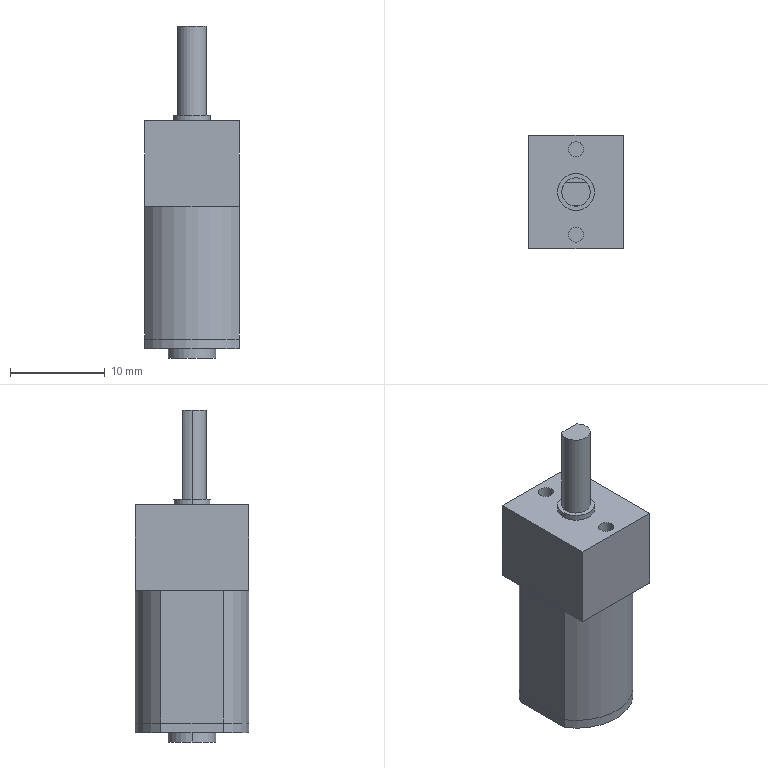Part | SolidWorks | features MBimport 1 | 4 solids | 39 faces | box 10 x 12 x 35 mm | volume 2719 mm3 | plane 23 | cylinder 16 | commonest cylinder face diameters 1.6 x4 3 x4 12 x4 3.9 x2 5 x2
STEP:
#1=CARTESIAN_POINT('',(5.,3.317,-14.));
#2=VERTEX_POINT('',#1);
#3=CARTESIAN_POINT('',(5.,-3.317,-14.));
#4=VERTEX_POINT('',#3);
#5=CARTESIAN_POINT('',(5.,1.658,-14.));
#6=DIRECTION('',(0.,-1.,0.));
#7=VECTOR('',#6,1000.);
#8=LINE('',#5,#7);
#9=EDGE_CURVE('',#2,#4,#8,.T.);
#10=ORIENTED_EDGE('',*,*,#9,.T.);
#11=CARTESIAN_POINT('',(-5.,-3.317,-14.));
#12=VERTEX_POINT('',#11);
#13=CARTESIAN_POINT('',(0.,0.,-14.));
#14=DIRECTION('',(0.,0.,-1.));
#15=DIRECTION('',(1.,0.,0.));
#16=AXIS2_PLACEMENT_3D('',#13,#14,#15);
#17=CIRCLE('',#16,6.);
#18=EDGE_CURVE('',#4,#12,#17,.T.);
#19=ORIENTED_EDGE('',*,*,#18,.T.);
#20=CARTESIAN_POINT('',(-5.,3.317,-14.));
#21=VERTEX_POINT('',#20);
#22=CARTESIAN_POINT('',(-5.,-1.658,-14.));
#23=DIRECTION('',(0.,1.,0.));
#24=VECTOR('',#23,1000.);
#25=LINE('',#22,#24);
#26=EDGE_CURVE('',#12,#21,#25,.T.);
#27=ORIENTED_EDGE('',*,*,#26,.T.);
#28=CARTESIAN_POINT('',(0.,0.,-14.));
#29=DIRECTION('',(0.,0.,-1.));
#30=DIRECTION('',(1.,0.,0.));
#31=AXIS2_PLACEMENT_3D('',#28,#29,#30);
#32=CIRCLE('',#31,6.);
#33=EDGE_CURVE('',#21,#2,#32,.T.);
#34=ORIENTED_EDGE('',*,*,#33,.T.);
#35=EDGE_LOOP('',(#10,#19,#27,#34));
#36=FACE_OUTER_BOUND('',#35,.T.);
#37=CARTESIAN_POINT('',(0.,0.,-14.));
#38=DIRECTION('',(0.,0.,-1.));
#39=DIRECTION('',(0.,-1.,0.));
#40=AXIS2_PLACEMENT_3D('',#37,#38,#39);
#41=PLANE('',#40);
#42=ADVANCED_FACE('',(#36),#41,.T.);
#43=ORIENTED_EDGE('',*,*,#18,.F.);
#44=CARTESIAN_POINT('',(5.,-3.317,0.));
#45=VERTEX_POINT('',#44);
#46=CARTESIAN_POINT('',(5.,-3.317,0.));
#47=DIRECTION('',(0.,0.,-1.));
#48=VECTOR('',#47,1000.);
#49=LINE('',#46,#48);
#50=EDGE_CURVE('',#45,#4,#49,.T.);
#51=ORIENTED_EDGE('',*,*,#50,.F.);
#52=CARTESIAN_POINT('',(-5.,-3.317,0.));
#53=VERTEX_POINT('',#52);
#54=CARTESIAN_POINT('',(0.,0.,0.));
#55=DIRECTION('',(0.,0.,1.));
#56=DIRECTION('',(1.,0.,0.));
#57=AXIS2_PLACEMENT_3D('',#54,#55,#56);
#58=CIRCLE('',#57,6.);
#59=EDGE_CURVE('',#53,#45,#58,.T.);
#60=ORIENTED_EDGE('',*,*,#59,.F.);
#61=CARTESIAN_POINT('',(-5.,-3.317,0.));
#62=DIRECTION('',(0.,0.,-1.));
#63=VECTOR('',#62,1000.);
#64=LINE('',#61,#63);
#65=EDGE_CURVE('',#53,#12,#64,.T.);
#66=ORIENTED_EDGE('',*,*,#65,.T.);
#67=EDGE_LOOP('',(#43,#51,#60,#66));
#68=FACE_OUTER_BOUND('',#67,.T.);
#69=CARTESIAN_POINT('',(0.,0.,0.));
#70=DIRECTION('',(0.,0.,-1.));
#71=DIRECTION('',(1.,0.,0.));
#72=AXIS2_PLACEMENT_3D('',#69,#70,#71);
#73=CYLINDRICAL_SURFACE('',#72,6.);
#74=ADVANCED_FACE('',(#68),#73,.T.);
#75=ORIENTED_EDGE('',*,*,#9,.F.);
#76=CARTESIAN_POINT('',(5.,3.317,0.));
#77=VERTEX_POINT('',#76);
#78=CARTESIAN_POINT('',(5.,3.317,0.));
#79=DIRECTION('',(0.,0.,-1.));
#80=VECTOR('',#79,1000.);
#81=LINE('',#78,#80);
#82=EDGE_CURVE('',#77,#2,#81,.T.);
#83=ORIENTED_EDGE('',*,*,#82,.F.);
#84=CARTESIAN_POINT('',(5.,6.,0.));
#85=DIRECTION('',(0.,-1.,0.));
#86=VECTOR('',#85,1000.);
#87=LINE('',#84,#86);
#88=EDGE_CURVE('',#77,#45,#87,.T.);
#89=ORIENTED_EDGE('',*,*,#88,.T.);
#90=ORIENTED_EDGE('',*,*,#50,.T.);
#91=EDGE_LOOP('',(#75,#83,#89,#90));
#92=FACE_OUTER_BOUND('',#91,.T.);
#93=CARTESIAN_POINT('',(5.,3.317,0.));
#94=DIRECTION('',(1.,0.,0.));
#95=DIRECTION('',(0.,1.,0.));
#96=AXIS2_PLACEMENT_3D('',#93,#94,#95);
#97=PLANE('',#96);
#98=ADVANCED_FACE('',(#92),#97,.T.);
#99=ORIENTED_EDGE('',*,*,#33,.F.);
#100=CARTESIAN_POINT('',(-5.,3.317,0.));
#101=VERTEX_POINT('',#100);
#102=CARTESIAN_POINT('',(-5.,3.317,0.));
#103=DIRECTION('',(0.,0.,-1.));
#104=VECTOR('',#103,1000.);
#105=LINE('',#102,#104);
#106=EDGE_CURVE('',#101,#21,#105,.T.);
#107=ORIENTED_EDGE('',*,*,#106,.F.);
#108=CARTESIAN_POINT('',(0.,0.,0.));
#109=DIRECTION('',(0.,0.,1.));
#110=DIRECTION('',(1.,0.,0.));
#111=AXIS2_PLACEMENT_3D('',#108,#109,#110);
#112=CIRCLE('',#111,6.);
#113=EDGE_CURVE('',#77,#101,#112,.T.);
#114=ORIENTED_EDGE('',*,*,#113,.F.);
#115=ORIENTED_EDGE('',*,*,#82,.T.);
#116=EDGE_LOOP('',(#99,#107,#114,#115));
#117=FACE_OUTER_BOUND('',#116,.T.);
#118=CARTESIAN_POINT('',(0.,0.,0.));
#119=DIRECTION('',(0.,0.,-1.));
#120=DIRECTION('',(1.,0.,0.));
#121=AXIS2_PLACEMENT_3D('',#118,#119,#120);
#122=CYLINDRICAL_SURFACE('',#121,6.);
#123=ADVANCED_FACE('',(#117),#122,.T.);
#124=ORIENTED_EDGE('',*,*,#26,.F.);
#125=ORIENTED_EDGE('',*,*,#65,.F.);
#126=CARTESIAN_POINT('',(-5.,-6.,0.));
#127=DIRECTION('',(0.,1.,0.));
#128=VECTOR('',#127,1000.);
#129=LINE('',#126,#128);
#130=EDGE_CURVE('',#53,#101,#129,.T.);
#131=ORIENTED_EDGE('',*,*,#130,.T.);
#132=ORIENTED_EDGE('',*,*,#106,.T.);
#133=EDGE_LOOP('',(#124,#125,#131,#132));
#134=FACE_OUTER_BOUND('',#133,.T.);
#135=CARTESIAN_POINT('',(-5.,-3.317,0.));
#136=DIRECTION('',(-1.,0.,0.));
#137=DIRECTION('',(0.,0.,1.));
#138=AXIS2_PLACEMENT_3D('',#135,#136,#137);
#139=PLANE('',#138);
#140=ADVANCED_FACE('',(#134),#139,.T.);
#141=ORIENTED_EDGE('',*,*,#59,.T.);
#142=ORIENTED_EDGE('',*,*,#88,.F.);
#143=ORIENTED_EDGE('',*,*,#113,.T.);
#144=ORIENTED_EDGE('',*,*,#130,.F.);
#145=EDGE_LOOP('',(#141,#142,#143,#144));
#146=FACE_OUTER_BOUND('',#145,.T.);
#147=CARTESIAN_POINT('',(0.,0.,0.));
#148=DIRECTION('',(0.,0.,1.));
#149=DIRECTION('',(1.,0.,0.));
#150=AXIS2_PLACEMENT_3D('',#147,#148,#149);
#151=PLANE('',#150);
#152=ADVANCED_FACE('',(#146),#151,.T.);
#153=CLOSED_SHELL('',(#42,#74,#98,#123,#140,#152));
#154=MANIFOLD_SOLID_BREP('',#153);
#155=CARTESIAN_POINT('',(1.5,0.,9.));
#156=VERTEX_POINT('',#155);
#157=CARTESIAN_POINT('',(-1.5,0.,9.));
#158=VERTEX_POINT('',#157);
#159=CARTESIAN_POINT('',(0.,0.,9.));
#160=DIRECTION('',(0.,0.,1.));
#161=DIRECTION('',(1.,0.,0.));
#162=AXIS2_PLACEMENT_3D('',#159,#160,#161);
#163=CIRCLE('',#162,1.5);
#164=EDGE_CURVE('',#156,#158,#163,.T.);
#165=ORIENTED_EDGE('',*,*,#164,.T.);
#166=CARTESIAN_POINT('',(-1.5,0.,19.));
#167=VERTEX_POINT('',#166);
#168=CARTESIAN_POINT('',(-1.5,0.,9.));
#169=DIRECTION('',(0.,0.,1.));
#170=VECTOR('',#169,1000.);
#171=LINE('',#168,#170);
#172=EDGE_CURVE('',#158,#167,#171,.T.);
#173=ORIENTED_EDGE('',*,*,#172,.T.);
#174=CARTESIAN_POINT('',(-1.118,1.,19.));
#175=VERTEX_POINT('',#174);
#176=CARTESIAN_POINT('',(0.,0.,19.));
#177=DIRECTION('',(0.,0.,1.));
#178=DIRECTION('',(1.,0.,0.));
#179=AXIS2_PLACEMENT_3D('',#176,#177,#178);
#180=CIRCLE('',#179,1.5);
#181=EDGE_CURVE('',#175,#167,#180,.T.);
#182=ORIENTED_EDGE('',*,*,#181,.F.);
#183=CARTESIAN_POINT('',(-1.118,1.,9.6));
#184=VERTEX_POINT('',#183);
#185=CARTESIAN_POINT('',(-1.118,1.,9.));
#186=DIRECTION('',(0.,0.,1.));
#187=VECTOR('',#186,1000.);
#188=LINE('',#185,#187);
#189=EDGE_CURVE('',#184,#175,#188,.T.);
#190=ORIENTED_EDGE('',*,*,#189,.F.);
#191=CARTESIAN_POINT('',(1.118,1.,9.6));
#192=VERTEX_POINT('',#191);
#193=CARTESIAN_POINT('',(0.,0.,9.6));
#194=DIRECTION('',(0.,0.,1.));
#195=DIRECTION('',(1.,0.,0.));
#196=AXIS2_PLACEMENT_3D('',#193,#194,#195);
#197=CIRCLE('',#196,1.5);
#198=EDGE_CURVE('',#192,#184,#197,.T.);
#199=ORIENTED_EDGE('',*,*,#198,.F.);
#200=CARTESIAN_POINT('',(1.118,1.,19.));
#201=VERTEX_POINT('',#200);
#202=CARTESIAN_POINT('',(1.118,1.,9.));
#203=DIRECTION('',(0.,0.,1.));
#204=VECTOR('',#203,1000.);
#205=LINE('',#202,#204);
#206=EDGE_CURVE('',#192,#201,#205,.T.);
#207=ORIENTED_EDGE('',*,*,#206,.T.);
#208=CARTESIAN_POINT('',(1.5,0.,19.));
#209=VERTEX_POINT('',#208);
#210=CARTESIAN_POINT('',(0.,0.,19.));
#211=DIRECTION('',(0.,0.,1.));
#212=DIRECTION('',(1.,0.,0.));
#213=AXIS2_PLACEMENT_3D('',#210,#211,#212);
#214=CIRCLE('',#213,1.5);
#215=EDGE_CURVE('',#209,#201,#214,.T.);
#216=ORIENTED_EDGE('',*,*,#215,.F.);
#217=CARTESIAN_POINT('',(1.5,0.,9.));
#218=DIRECTION('',(0.,0.,1.));
#219=VECTOR('',#218,1000.);
#220=LINE('',#217,#219);
#221=EDGE_CURVE('',#156,#209,#220,.T.);
#222=ORIENTED_EDGE('',*,*,#221,.F.);
#223=EDGE_LOOP('',(#165,#173,#182,#190,#199,#207,#216,#222));
#224=FACE_OUTER_BOUND('',#223,.T.);
#225=CARTESIAN_POINT('',(0.,0.,9.));
#226=DIRECTION('',(0.,0.,1.));
#227=DIRECTION('',(1.,0.,0.));
#228=AXIS2_PLACEMENT_3D('',#225,#226,#227);
#229=CYLINDRICAL_SURFACE('',#228,1.5);
#230=ADVANCED_FACE('',(#224),#229,.T.);
#231=ORIENTED_EDGE('',*,*,#164,.F.);
#232=CARTESIAN_POINT('',(0.,0.,9.));
#233=DIRECTION('',(0.,0.,1.));
#234=DIRECTION('',(1.,0.,0.));
#235=AXIS2_PLACEMENT_3D('',#232,#233,#234);
#236=CIRCLE('',#235,1.5);
#237=EDGE_CURVE('',#158,#156,#236,.T.);
#238=ORIENTED_EDGE('',*,*,#237,.F.);
#239=EDGE_LOOP('',(#231,#238));
#240=FACE_OUTER_BOUND('',#239,.T.);
#241=CARTESIAN_POINT('',(0.,1.25,9.));
#242=DIRECTION('',(0.,0.,1.));
#243=DIRECTION('',(1.,0.,0.));
#244=AXIS2_PLACEMENT_3D('',#241,#242,#243);
#245=PLANE('',#244);
#246=ADVANCED_FACE('',(#240),#245,.F.);
#247=ORIENTED_EDGE('',*,*,#198,.T.);
#248=CARTESIAN_POINT('',(1.118,1.,9.6));
#249=DIRECTION('',(1.,0.,0.));
#250=VECTOR('',#249,1000.);
#251=LINE('',#248,#250);
#252=EDGE_CURVE('',#184,#192,#251,.T.);
#253=ORIENTED_EDGE('',*,*,#252,.T.);
#254=EDGE_LOOP('',(#247,#253));
#255=FACE_OUTER_BOUND('',#254,.T.);
#256=CARTESIAN_POINT('',(0.,1.25,9.6));
#257=DIRECTION('',(0.,0.,1.));
#258=DIRECTION('',(1.,0.,0.));
#259=AXIS2_PLACEMENT_3D('',#256,#257,#258);
#260=PLANE('',#259);
#261=ADVANCED_FACE('',(#255),#260,.T.);
#262=ORIENTED_EDGE('',*,*,#172,.F.);
#263=ORIENTED_EDGE('',*,*,#237,.T.);
#264=ORIENTED_EDGE('',*,*,#221,.T.);
#265=CARTESIAN_POINT('',(0.,0.,19.));
#266=DIRECTION('',(0.,0.,1.));
#267=DIRECTION('',(1.,0.,0.));
#268=AXIS2_PLACEMENT_3D('',#265,#266,#267);
#269=CIRCLE('',#268,1.5);
#270=EDGE_CURVE('',#167,#209,#269,.T.);
#271=ORIENTED_EDGE('',*,*,#270,.F.);
#272=EDGE_LOOP('',(#262,#263,#264,#271));
#273=FACE_OUTER_BOUND('',#272,.T.);
#274=CARTESIAN_POINT('',(0.,0.,9.));
#275=DIRECTION('',(0.,0.,1.));
#276=DIRECTION('',(1.,0.,0.));
#277=AXIS2_PLACEMENT_3D('',#274,#275,#276);
#278=CYLINDRICAL_SURFACE('',#277,1.5);
#279=ADVANCED_FACE('',(#273),#278,.T.);
#280=CARTESIAN_POINT('',(1.118,1.,19.));
#281=DIRECTION('',(-1.,0.,0.));
#282=VECTOR('',#281,1000.);
#283=LINE('',#280,#282);
#284=EDGE_CURVE('',#201,#175,#283,.T.);
#285=ORIENTED_EDGE('',*,*,#284,.T.);
#286=ORIENTED_EDGE('',*,*,#181,.T.);
#287=ORIENTED_EDGE('',*,*,#270,.T.);
#288=ORIENTED_EDGE('',*,*,#215,.T.);
#289=EDGE_LOOP('',(#285,#286,#287,#288));
#290=FACE_OUTER_BOUND('',#289,.T.);
#291=CARTESIAN_POINT('',(0.,-0.25,19.));
#292=DIRECTION('',(0.,0.,1.));
#293=DIRECTION('',(1.,0.,0.));
#294=AXIS2_PLACEMENT_3D('',#291,#292,#293);
#295=PLANE('',#294);
#296=ADVANCED_FACE('',(#290),#295,.T.);
#297=ORIENTED_EDGE('',*,*,#252,.F.);
#298=ORIENTED_EDGE('',*,*,#189,.T.);
#299=ORIENTED_EDGE('',*,*,#284,.F.);
#300=ORIENTED_EDGE('',*,*,#206,.F.);
#301=EDGE_LOOP('',(#297,#298,#299,#300));
#302=FACE_OUTER_BOUND('',#301,.T.);
#303=CARTESIAN_POINT('',(1.118,1.,9.));
#304=DIRECTION('',(0.,1.,0.));
#305=DIRECTION('',(1.,0.,0.));
#306=AXIS2_PLACEMENT_3D('',#303,#304,#305);
#307=PLANE('',#306);
#308=ADVANCED_FACE('',(#302),#307,.T.);
#309=CLOSED_SHELL('',(#230,#246,#261,#279,#296,#308));
#310=MANIFOLD_SOLID_BREP('',#309);
#311=CARTESIAN_POINT('',(2.5,0.,-15.));
#312=VERTEX_POINT('',#311);
#313=CARTESIAN_POINT('',(-2.5,0.,-15.));
#314=VERTEX_POINT('',#313);
#315=CARTESIAN_POINT('',(0.,0.,-15.));
#316=DIRECTION('',(0.,0.,1.));
#317=DIRECTION('',(-1.,0.,0.));
#318=AXIS2_PLACEMENT_3D('',#315,#316,#317);
#319=CIRCLE('',#318,2.5);
#320=EDGE_CURVE('',#312,#314,#319,.T.);
#321=ORIENTED_EDGE('',*,*,#320,.F.);
#322=CARTESIAN_POINT('',(2.5,0.,-16.));
#323=VERTEX_POINT('',#322);
#324=CARTESIAN_POINT('',(2.5,0.,-15.));
#325=DIRECTION('',(0.,0.,-1.));
#326=VECTOR('',#325,1000.);
#327=LINE('',#324,#326);
#328=EDGE_CURVE('',#312,#323,#327,.T.);
#329=ORIENTED_EDGE('',*,*,#328,.T.);
#330=CARTESIAN_POINT('',(-2.5,0.,-16.));
#331=VERTEX_POINT('',#330);
#332=CARTESIAN_POINT('',(0.,0.,-16.));
#333=DIRECTION('',(0.,0.,-1.));
#334=DIRECTION('',(-1.,0.,0.));
#335=AXIS2_PLACEMENT_3D('',#332,#333,#334);
#336=CIRCLE('',#335,2.5);
#337=EDGE_CURVE('',#331,#323,#336,.T.);
#338=ORIENTED_EDGE('',*,*,#337,.F.);
#339=CARTESIAN_POINT('',(-2.5,0.,-15.));
#340=DIRECTION('',(0.,0.,-1.));
#341=VECTOR('',#340,1000.);
#342=LINE('',#339,#341);
#343=EDGE_CURVE('',#314,#331,#342,.T.);
#344=ORIENTED_EDGE('',*,*,#343,.F.);
#345=EDGE_LOOP('',(#321,#329,#338,#344));
#346=FACE_OUTER_BOUND('',#345,.T.);
#347=CARTESIAN_POINT('',(0.,0.,-15.));
#348=DIRECTION('',(0.,0.,-1.));
#349=DIRECTION('',(-1.,0.,0.));
#350=AXIS2_PLACEMENT_3D('',#347,#348,#349);
#351=CYLINDRICAL_SURFACE('',#350,2.5);
#352=ADVANCED_FACE('',(#346),#351,.T.);
#353=CARTESIAN_POINT('',(0.,0.,-15.));
#354=DIRECTION('',(0.,0.,1.));
#355=DIRECTION('',(-1.,0.,0.));
#356=AXIS2_PLACEMENT_3D('',#353,#354,#355);
#357=CIRCLE('',#356,2.5);
#358=EDGE_CURVE('',#314,#312,#357,.T.);
#359=ORIENTED_EDGE('',*,*,#358,.T.);
#360=ORIENTED_EDGE('',*,*,#320,.T.);
#361=EDGE_LOOP('',(#359,#360));
#362=FACE_BOUND('',#361,.T.);
#363=CARTESIAN_POINT('',(5.,-3.317,-15.));
#364=VERTEX_POINT('',#363);
#365=CARTESIAN_POINT('',(-5.,-3.317,-15.));
#366=VERTEX_POINT('',#365);
#367=CARTESIAN_POINT('',(0.,0.,-15.));
#368=DIRECTION('',(0.,0.,-1.));
#369=DIRECTION('',(1.,0.,0.));
#370=AXIS2_PLACEMENT_3D('',#367,#368,#369);
#371=CIRCLE('',#370,6.);
#372=EDGE_CURVE('',#364,#366,#371,.T.);
#373=ORIENTED_EDGE('',*,*,#372,.T.);
#374=CARTESIAN_POINT('',(-5.,3.317,-15.));
#375=VERTEX_POINT('',#374);
#376=CARTESIAN_POINT('',(-5.,-6.,-15.));
#377=DIRECTION('',(0.,1.,0.));
#378=VECTOR('',#377,1000.);
#379=LINE('',#376,#378);
#380=EDGE_CURVE('',#366,#375,#379,.T.);
#381=ORIENTED_EDGE('',*,*,#380,.T.);
#382=CARTESIAN_POINT('',(5.,3.317,-15.));
#383=VERTEX_POINT('',#382);
#384=CARTESIAN_POINT('',(0.,0.,-15.));
#385=DIRECTION('',(0.,0.,-1.));
#386=DIRECTION('',(1.,0.,0.));
#387=AXIS2_PLACEMENT_3D('',#384,#385,#386);
#388=CIRCLE('',#387,6.);
#389=EDGE_CURVE('',#375,#383,#388,.T.);
#390=ORIENTED_EDGE('',*,*,#389,.T.);
#391=CARTESIAN_POINT('',(5.,6.,-15.));
#392=DIRECTION('',(0.,-1.,0.));
#393=VECTOR('',#392,1000.);
#394=LINE('',#391,#393);
#395=EDGE_CURVE('',#383,#364,#394,.T.);
#396=ORIENTED_EDGE('',*,*,#395,.T.);
#397=EDGE_LOOP('',(#373,#381,#390,#396));
#398=FACE_OUTER_BOUND('',#397,.T.);
#399=CARTESIAN_POINT('',(0.,0.,-15.));
#400=DIRECTION('',(0.,0.,1.));
#401=DIRECTION('',(1.,0.,0.));
#402=AXIS2_PLACEMENT_3D('',#399,#400,#401);
#403=PLANE('',#402);
#404=ADVANCED_FACE('',(#362,#398),#403,.F.);
#405=CARTESIAN_POINT('',(5.,-3.317,-14.));
#406=VERTEX_POINT('',#405);
#407=CARTESIAN_POINT('',(-5.,-3.317,-14.));
#408=VERTEX_POINT('',#407);
#409=CARTESIAN_POINT('',(0.,0.,-14.));
#410=DIRECTION('',(0.,0.,-1.));
#411=DIRECTION('',(1.,0.,0.));
#412=AXIS2_PLACEMENT_3D('',#409,#410,#411);
#413=CIRCLE('',#412,6.);
#414=EDGE_CURVE('',#406,#408,#413,.T.);
#415=ORIENTED_EDGE('',*,*,#414,.T.);
#416=CARTESIAN_POINT('',(-5.,-3.317,0.));
#417=DIRECTION('',(0.,0.,-1.));
#418=VECTOR('',#417,1000.);
#419=LINE('',#416,#418);
#420=EDGE_CURVE('',#408,#366,#419,.T.);
#421=ORIENTED_EDGE('',*,*,#420,.T.);
#422=ORIENTED_EDGE('',*,*,#372,.F.);
#423=CARTESIAN_POINT('',(5.,-3.317,0.));
#424=DIRECTION('',(0.,0.,-1.));
#425=VECTOR('',#424,1000.);
#426=LINE('',#423,#425);
#427=EDGE_CURVE('',#406,#364,#426,.T.);
#428=ORIENTED_EDGE('',*,*,#427,.F.);
#429=EDGE_LOOP('',(#415,#421,#422,#428));
#430=FACE_OUTER_BOUND('',#429,.T.);
#431=CARTESIAN_POINT('',(0.,0.,0.));
#432=DIRECTION('',(0.,0.,-1.));
#433=DIRECTION('',(1.,0.,0.));
#434=AXIS2_PLACEMENT_3D('',#431,#432,#433);
#435=CYLINDRICAL_SURFACE('',#434,6.);
#436=ADVANCED_FACE('',(#430),#435,.T.);
#437=CARTESIAN_POINT('',(5.,3.317,-14.));
#438=VERTEX_POINT('',#437);
#439=CARTESIAN_POINT('',(5.,1.658,-14.));
#440=DIRECTION('',(0.,-1.,0.));
#441=VECTOR('',#440,1000.);
#442=LINE('',#439,#441);
#443=EDGE_CURVE('',#438,#406,#442,.T.);
#444=ORIENTED_EDGE('',*,*,#443,.T.);
#445=ORIENTED_EDGE('',*,*,#427,.T.);
#446=ORIENTED_EDGE('',*,*,#395,.F.);
#447=CARTESIAN_POINT('',(5.,3.317,0.));
#448=DIRECTION('',(0.,0.,-1.));
#449=VECTOR('',#448,1000.);
#450=LINE('',#447,#449);
#451=EDGE_CURVE('',#438,#383,#450,.T.);
#452=ORIENTED_EDGE('',*,*,#451,.F.);
#453=EDGE_LOOP('',(#444,#445,#446,#452));
#454=FACE_OUTER_BOUND('',#453,.T.);
#455=CARTESIAN_POINT('',(5.,3.317,0.));
#456=DIRECTION('',(1.,0.,0.));
#457=DIRECTION('',(0.,1.,0.));
#458=AXIS2_PLACEMENT_3D('',#455,#456,#457);
#459=PLANE('',#458);
#460=ADVANCED_FACE('',(#454),#459,.T.);
#461=ORIENTED_EDGE('',*,*,#337,.T.);
#462=CARTESIAN_POINT('',(0.,0.,-16.));
#463=DIRECTION('',(0.,0.,-1.));
#464=DIRECTION('',(-1.,0.,0.));
#465=AXIS2_PLACEMENT_3D('',#462,#463,#464);
#466=CIRCLE('',#465,2.5);
#467=EDGE_CURVE('',#323,#331,#466,.T.);
#468=ORIENTED_EDGE('',*,*,#467,.T.);
#469=EDGE_LOOP('',(#461,#468));
#470=FACE_OUTER_BOUND('',#469,.T.);
#471=CARTESIAN_POINT('',(0.,0.,-16.));
#472=DIRECTION('',(0.,0.,-1.));
#473=DIRECTION('',(0.,-1.,0.));
#474=AXIS2_PLACEMENT_3D('',#471,#472,#473);
#475=PLANE('',#474);
#476=ADVANCED_FACE('',(#470),#475,.T.);
#477=ORIENTED_EDGE('',*,*,#328,.F.);
#478=ORIENTED_EDGE('',*,*,#358,.F.);
#479=ORIENTED_EDGE('',*,*,#343,.T.);
#480=ORIENTED_EDGE('',*,*,#467,.F.);
#481=EDGE_LOOP('',(#477,#478,#479,#480));
#482=FACE_OUTER_BOUND('',#481,.T.);
#483=CARTESIAN_POINT('',(0.,0.,-15.));
#484=DIRECTION('',(0.,0.,-1.));
#485=DIRECTION('',(-1.,0.,0.));
#486=AXIS2_PLACEMENT_3D('',#483,#484,#485);
#487=CYLINDRICAL_SURFACE('',#486,2.5);
#488=ADVANCED_FACE('',(#482),#487,.T.);
#489=CARTESIAN_POINT('',(-5.,3.317,-14.));
#490=VERTEX_POINT('',#489);
#491=CARTESIAN_POINT('',(0.,0.,-14.));
#492=DIRECTION('',(0.,0.,-1.));
#493=DIRECTION('',(1.,0.,0.));
#494=AXIS2_PLACEMENT_3D('',#491,#492,#493);
#495=CIRCLE('',#494,6.);
#496=EDGE_CURVE('',#490,#438,#495,.T.);
#497=ORIENTED_EDGE('',*,*,#496,.T.);
#498=ORIENTED_EDGE('',*,*,#451,.T.);
#499=ORIENTED_EDGE('',*,*,#389,.F.);
#500=CARTESIAN_POINT('',(-5.,3.317,0.));
#501=DIRECTION('',(0.,0.,-1.));
#502=VECTOR('',#501,1000.);
#503=LINE('',#500,#502);
#504=EDGE_CURVE('',#490,#375,#503,.T.);
#505=ORIENTED_EDGE('',*,*,#504,.F.);
#506=EDGE_LOOP('',(#497,#498,#499,#505));
#507=FACE_OUTER_BOUND('',#506,.T.);
#508=CARTESIAN_POINT('',(0.,0.,0.));
#509=DIRECTION('',(0.,0.,-1.));
#510=DIRECTION('',(1.,0.,0.));
#511=AXIS2_PLACEMENT_3D('',#508,#509,#510);
#512=CYLINDRICAL_SURFACE('',#511,6.);
#513=ADVANCED_FACE('',(#507),#512,.T.);
#514=CARTESIAN_POINT('',(-5.,-1.658,-14.));
#515=DIRECTION('',(0.,1.,0.));
#516=VECTOR('',#515,1000.);
#517=LINE('',#514,#516);
#518=EDGE_CURVE('',#408,#490,#517,.T.);
#519=ORIENTED_EDGE('',*,*,#518,.T.);
#520=ORIENTED_EDGE('',*,*,#504,.T.);
#521=ORIENTED_EDGE('',*,*,#380,.F.);
#522=ORIENTED_EDGE('',*,*,#420,.F.);
#523=EDGE_LOOP('',(#519,#520,#521,#522));
#524=FACE_OUTER_BOUND('',#523,.T.);
#525=CARTESIAN_POINT('',(-5.,-3.317,0.));
#526=DIRECTION('',(-1.,0.,0.));
#527=DIRECTION('',(0.,0.,1.));
#528=AXIS2_PLACEMENT_3D('',#525,#526,#527);
#529=PLANE('',#528);
#530=ADVANCED_FACE('',(#524),#529,.T.);
#531=ORIENTED_EDGE('',*,*,#443,.F.);
#532=ORIENTED_EDGE('',*,*,#496,.F.);
#533=ORIENTED_EDGE('',*,*,#518,.F.);
#534=ORIENTED_EDGE('',*,*,#414,.F.);
#535=EDGE_LOOP('',(#531,#532,#533,#534));
#536=FACE_OUTER_BOUND('',#535,.T.);
#537=CARTESIAN_POINT('',(0.,0.,-14.));
#538=DIRECTION('',(0.,0.,-1.));
#539=DIRECTION('',(0.,-1.,0.));
#540=AXIS2_PLACEMENT_3D('',#537,#538,#539);
#541=PLANE('',#540);
#542=ADVANCED_FACE('',(#536),#541,.F.);
#543=CLOSED_SHELL('',(#352,#404,#436,#460,#476,#488,#513,#530,#542));
#544=MANIFOLD_SOLID_BREP('',#543);
#545=CARTESIAN_POINT('',(-0.8,4.5,9.));
#546=VERTEX_POINT('',#545);
#547=CARTESIAN_POINT('',(0.8,4.5,9.));
#548=VERTEX_POINT('',#547);
#549=CARTESIAN_POINT('',(0.,4.5,9.));
#550=DIRECTION('',(0.,0.,-1.));
#551=DIRECTION('',(1.,0.,0.));
#552=AXIS2_PLACEMENT_3D('',#549,#550,#551);
#553=CIRCLE('',#552,0.8);
#554=EDGE_CURVE('',#546,#548,#553,.T.);
#555=ORIENTED_EDGE('',*,*,#554,.F.);
#556=CARTESIAN_POINT('',(-0.8,4.5,7.));
#557=VERTEX_POINT('',#556);
#558=CARTESIAN_POINT('',(-0.8,4.5,9.));
#559=DIRECTION('',(0.,0.,-1.));
#560=VECTOR('',#559,1000.);
#561=LINE('',#558,#560);
#562=EDGE_CURVE('',#546,#557,#561,.T.);
#563=ORIENTED_EDGE('',*,*,#562,.T.);
#564=CARTESIAN_POINT('',(0.8,4.5,7.));
#565=VERTEX_POINT('',#564);
#566=CARTESIAN_POINT('',(0.,4.5,7.));
#567=DIRECTION('',(0.,0.,-1.));
#568=DIRECTION('',(1.,0.,0.));
#569=AXIS2_PLACEMENT_3D('',#566,#567,#568);
#570=CIRCLE('',#569,0.8);
#571=EDGE_CURVE('',#557,#565,#570,.T.);
#572=ORIENTED_EDGE('',*,*,#571,.T.);
#573=CARTESIAN_POINT('',(0.8,4.5,9.));
#574=DIRECTION('',(0.,0.,-1.));
#575=VECTOR('',#574,1000.);
#576=LINE('',#573,#575);
#577=EDGE_CURVE('',#548,#565,#576,.T.);
#578=ORIENTED_EDGE('',*,*,#577,.F.);
#579=EDGE_LOOP('',(#555,#563,#572,#578));
#580=FACE_OUTER_BOUND('',#579,.T.);
#581=CARTESIAN_POINT('',(0.,4.5,9.));
#582=DIRECTION('',(0.,0.,-1.));
#583=DIRECTION('',(1.,0.,0.));
#584=AXIS2_PLACEMENT_3D('',#581,#582,#583);
#585=CYLINDRICAL_SURFACE('',#584,0.8);
#586=ADVANCED_FACE('',(#580),#585,.F.);
#587=CARTESIAN_POINT('',(-0.8,-4.5,9.));
#588=VERTEX_POINT('',#587);
#589=CARTESIAN_POINT('',(0.8,-4.5,9.));
#590=VERTEX_POINT('',#589);
#591=CARTESIAN_POINT('',(0.,-4.5,9.));
#592=DIRECTION('',(0.,0.,-1.));
#593=DIRECTION('',(1.,0.,0.));
#594=AXIS2_PLACEMENT_3D('',#591,#592,#593);
#595=CIRCLE('',#594,0.8);
#596=EDGE_CURVE('',#588,#590,#595,.T.);
#597=ORIENTED_EDGE('',*,*,#596,.F.);
#598=CARTESIAN_POINT('',(-0.8,-4.5,7.));
#599=VERTEX_POINT('',#598);
#600=CARTESIAN_POINT('',(-0.8,-4.5,9.));
#601=DIRECTION('',(0.,0.,-1.));
#602=VECTOR('',#601,1000.);
#603=LINE('',#600,#602);
#604=EDGE_CURVE('',#588,#599,#603,.T.);
#605=ORIENTED_EDGE('',*,*,#604,.T.);
#606=CARTESIAN_POINT('',(0.8,-4.5,7.));
#607=VERTEX_POINT('',#606);
#608=CARTESIAN_POINT('',(0.,-4.5,7.));
#609=DIRECTION('',(0.,0.,-1.));
#610=DIRECTION('',(1.,0.,0.));
#611=AXIS2_PLACEMENT_3D('',#608,#609,#610);
#612=CIRCLE('',#611,0.8);
#613=EDGE_CURVE('',#599,#607,#612,.T.);
#614=ORIENTED_EDGE('',*,*,#613,.T.);
#615=CARTESIAN_POINT('',(0.8,-4.5,9.));
#616=DIRECTION('',(0.,0.,-1.));
#617=VECTOR('',#616,1000.);
#618=LINE('',#615,#617);
#619=EDGE_CURVE('',#590,#607,#618,.T.);
#620=ORIENTED_EDGE('',*,*,#619,.F.);
#621=EDGE_LOOP('',(#597,#605,#614,#620));
#622=FACE_OUTER_BOUND('',#621,.T.);
#623=CARTESIAN_POINT('',(0.,-4.5,9.));
#624=DIRECTION('',(0.,0.,-1.));
#625=DIRECTION('',(1.,0.,0.));
#626=AXIS2_PLACEMENT_3D('',#623,#624,#625);
#627=CYLINDRICAL_SURFACE('',#626,0.8);
#628=ADVANCED_FACE('',(#622),#627,.F.);
#629=CARTESIAN_POINT('',(-1.5,0.,9.));
#630=VERTEX_POINT('',#629);
#631=CARTESIAN_POINT('',(1.5,0.,9.));
#632=VERTEX_POINT('',#631);
#633=CARTESIAN_POINT('',(0.,0.,9.));
#634=DIRECTION('',(0.,0.,1.));
#635=DIRECTION('',(1.,0.,0.));
#636=AXIS2_PLACEMENT_3D('',#633,#634,#635);
#637=CIRCLE('',#636,1.5);
#638=EDGE_CURVE('',#630,#632,#637,.T.);
#639=ORIENTED_EDGE('',*,*,#638,.F.);
#640=CARTESIAN_POINT('',(-1.5,0.,9.6));
#641=VERTEX_POINT('',#640);
#642=CARTESIAN_POINT('',(-1.5,0.,9.));
#643=DIRECTION('',(0.,0.,1.));
#644=VECTOR('',#643,1000.);
#645=LINE('',#642,#644);
#646=EDGE_CURVE('',#630,#641,#645,.T.);
#647=ORIENTED_EDGE('',*,*,#646,.T.);
#648=CARTESIAN_POINT('',(1.5,0.,9.6));
#649=VERTEX_POINT('',#648);
#650=CARTESIAN_POINT('',(0.,0.,9.6));
#651=DIRECTION('',(0.,0.,-1.));
#652=DIRECTION('',(1.,0.,0.));
#653=AXIS2_PLACEMENT_3D('',#650,#651,#652);
#654=CIRCLE('',#653,1.5);
#655=EDGE_CURVE('',#649,#641,#654,.T.);
#656=ORIENTED_EDGE('',*,*,#655,.F.);
#657=CARTESIAN_POINT('',(1.5,0.,9.));
#658=DIRECTION('',(0.,0.,1.));
#659=VECTOR('',#658,1000.);
#660=LINE('',#657,#659);
#661=EDGE_CURVE('',#632,#649,#660,.T.);
#662=ORIENTED_EDGE('',*,*,#661,.F.);
#663=EDGE_LOOP('',(#639,#647,#656,#662));
#664=FACE_OUTER_BOUND('',#663,.T.);
#665=CARTESIAN_POINT('',(0.,0.,9.));
#666=DIRECTION('',(0.,0.,1.));
#667=DIRECTION('',(1.,0.,0.));
#668=AXIS2_PLACEMENT_3D('',#665,#666,#667);
#669=CYLINDRICAL_SURFACE('',#668,1.5);
#670=ADVANCED_FACE('',(#664),#669,.F.);
#671=CARTESIAN_POINT('',(-1.95,0.,9.));
#672=VERTEX_POINT('',#671);
#673=CARTESIAN_POINT('',(1.95,0.,9.));
#674=VERTEX_POINT('',#673);
#675=CARTESIAN_POINT('',(0.,0.,9.));
#676=DIRECTION('',(0.,0.,-1.));
#677=DIRECTION('',(1.,0.,0.));
#678=AXIS2_PLACEMENT_3D('',#675,#676,#677);
#679=CIRCLE('',#678,1.95);
#680=EDGE_CURVE('',#672,#674,#679,.T.);
#681=ORIENTED_EDGE('',*,*,#680,.F.);
#682=CARTESIAN_POINT('',(-1.95,0.,9.6));
#683=VERTEX_POINT('',#682);
#684=CARTESIAN_POINT('',(-1.95,0.,9.));
#685=DIRECTION('',(0.,0.,1.));
#686=VECTOR('',#685,1000.);
#687=LINE('',#684,#686);
#688=EDGE_CURVE('',#672,#683,#687,.T.);
#689=ORIENTED_EDGE('',*,*,#688,.T.);
#690=CARTESIAN_POINT('',(1.95,0.,9.6));
#691=VERTEX_POINT('',#690);
#692=CARTESIAN_POINT('',(0.,0.,9.6));
#693=DIRECTION('',(0.,0.,1.));
#694=DIRECTION('',(1.,0.,0.));
#695=AXIS2_PLACEMENT_3D('',#692,#693,#694);
#696=CIRCLE('',#695,1.95);
#697=EDGE_CURVE('',#691,#683,#696,.T.);
#698=ORIENTED_EDGE('',*,*,#697,.F.);
#699=CARTESIAN_POINT('',(1.95,0.,9.));
#700=DIRECTION('',(0.,0.,1.));
#701=VECTOR('',#700,1000.);
#702=LINE('',#699,#701);
#703=EDGE_CURVE('',#674,#691,#702,.T.);
#704=ORIENTED_EDGE('',*,*,#703,.F.);
#705=EDGE_LOOP('',(#681,#689,#698,#704));
#706=FACE_OUTER_BOUND('',#705,.T.);
#707=CARTESIAN_POINT('',(0.,0.,9.));
#708=DIRECTION('',(0.,0.,1.));
#709=DIRECTION('',(1.,0.,0.));
#710=AXIS2_PLACEMENT_3D('',#707,#708,#709);
#711=CYLINDRICAL_SURFACE('',#710,1.95);
#712=ADVANCED_FACE('',(#706),#711,.T.);
#713=CARTESIAN_POINT('',(5.,-6.,0.));
#714=VERTEX_POINT('',#713);
#715=CARTESIAN_POINT('',(-5.,-6.,0.));
#716=VERTEX_POINT('',#715);
#717=CARTESIAN_POINT('',(5.,-6.,0.));
#718=DIRECTION('',(-1.,0.,0.));
#719=VECTOR('',#718,1000.);
#720=LINE('',#717,#719);
#721=EDGE_CURVE('',#714,#716,#720,.T.);
#722=ORIENTED_EDGE('',*,*,#721,.T.);
#723=CARTESIAN_POINT('',(-5.,6.,0.));
#724=VERTEX_POINT('',#723);
#725=CARTESIAN_POINT('',(-5.,-6.,0.));
#726=DIRECTION('',(0.,1.,0.));
#727=VECTOR('',#726,1000.);
#728=LINE('',#725,#727);
#729=EDGE_CURVE('',#716,#724,#728,.T.);
#730=ORIENTED_EDGE('',*,*,#729,.T.);
#731=CARTESIAN_POINT('',(5.,6.,0.));
#732=VERTEX_POINT('',#731);
#733=CARTESIAN_POINT('',(-5.,6.,0.));
#734=DIRECTION('',(1.,0.,0.));
#735=VECTOR('',#734,1000.);
#736=LINE('',#733,#735);
#737=EDGE_CURVE('',#724,#732,#736,.T.);
#738=ORIENTED_EDGE('',*,*,#737,.T.);
#739=CARTESIAN_POINT('',(5.,6.,0.));
#740=DIRECTION('',(0.,-1.,0.));
#741=VECTOR('',#740,1000.);
#742=LINE('',#739,#741);
#743=EDGE_CURVE('',#732,#714,#742,.T.);
#744=ORIENTED_EDGE('',*,*,#743,.T.);
#745=EDGE_LOOP('',(#722,#730,#738,#744));
#746=FACE_OUTER_BOUND('',#745,.T.);
#747=CARTESIAN_POINT('',(0.,0.,0.));
#748=DIRECTION('',(0.,0.,1.));
#749=DIRECTION('',(1.,0.,0.));
#750=AXIS2_PLACEMENT_3D('',#747,#748,#749);
#751=PLANE('',#750);
#752=ADVANCED_FACE('',(#746),#751,.F.);
#753=CARTESIAN_POINT('',(0.,0.,9.));
#754=DIRECTION('',(0.,0.,1.));
#755=DIRECTION('',(1.,0.,0.));
#756=AXIS2_PLACEMENT_3D('',#753,#754,#755);
#757=CIRCLE('',#756,1.5);
#758=EDGE_CURVE('',#632,#630,#757,.T.);
#759=ORIENTED_EDGE('',*,*,#758,.T.);
#760=ORIENTED_EDGE('',*,*,#638,.T.);
#761=EDGE_LOOP('',(#759,#760));
#762=FACE_OUTER_BOUND('',#761,.T.);
#763=CARTESIAN_POINT('',(0.,0.,9.));
#764=DIRECTION('',(0.,0.,1.));
#765=DIRECTION('',(1.,0.,0.));
#766=AXIS2_PLACEMENT_3D('',#763,#764,#765);
#767=PLANE('',#766);
#768=ADVANCED_FACE('',(#762),#767,.T.);
#769=ORIENTED_EDGE('',*,*,#721,.F.);
#770=CARTESIAN_POINT('',(5.,-6.,9.));
#771=VERTEX_POINT('',#770);
#772=CARTESIAN_POINT('',(5.,-6.,0.));
#773=DIRECTION('',(0.,0.,1.));
#774=VECTOR('',#773,1000.);
#775=LINE('',#772,#774);
#776=EDGE_CURVE('',#714,#771,#775,.T.);
#777=ORIENTED_EDGE('',*,*,#776,.T.);
#778=CARTESIAN_POINT('',(-5.,-6.,9.));
#779=VERTEX_POINT('',#778);
#780=CARTESIAN_POINT('',(5.,-6.,9.));
#781=DIRECTION('',(1.,0.,0.));
#782=VECTOR('',#781,1000.);
#783=LINE('',#780,#782);
#784=EDGE_CURVE('',#779,#771,#783,.T.);
#785=ORIENTED_EDGE('',*,*,#784,.F.);
#786=CARTESIAN_POINT('',(-5.,-6.,0.));
#787=DIRECTION('',(0.,0.,1.));
#788=VECTOR('',#787,1000.);
#789=LINE('',#786,#788);
#790=EDGE_CURVE('',#716,#779,#789,.T.);
#791=ORIENTED_EDGE('',*,*,#790,.F.);
#792=EDGE_LOOP('',(#769,#777,#785,#791));
#793=FACE_OUTER_BOUND('',#792,.T.);
#794=CARTESIAN_POINT('',(-5.,-6.,0.));
#795=DIRECTION('',(0.,-1.,0.));
#796=DIRECTION('',(0.,0.,-1.));
#797=AXIS2_PLACEMENT_3D('',#794,#795,#796);
#798=PLANE('',#797);
#799=ADVANCED_FACE('',(#793),#798,.T.);
#800=ORIENTED_EDGE('',*,*,#743,.F.);
#801=CARTESIAN_POINT('',(5.,6.,9.));
#802=VERTEX_POINT('',#801);
#803=CARTESIAN_POINT('',(5.,6.,0.));
#804=DIRECTION('',(0.,0.,1.));
#805=VECTOR('',#804,1000.);
#806=LINE('',#803,#805);
#807=EDGE_CURVE('',#732,#802,#806,.T.);
#808=ORIENTED_EDGE('',*,*,#807,.T.);
#809=CARTESIAN_POINT('',(5.,6.,9.));
#810=DIRECTION('',(0.,1.,0.));
#811=VECTOR('',#810,1000.);
#812=LINE('',#809,#811);
#813=EDGE_CURVE('',#771,#802,#812,.T.);
#814=ORIENTED_EDGE('',*,*,#813,.F.);
#815=ORIENTED_EDGE('',*,*,#776,.F.);
#816=EDGE_LOOP('',(#800,#808,#814,#815));
#817=FACE_OUTER_BOUND('',#816,.T.);
#818=CARTESIAN_POINT('',(5.,-6.,0.));
#819=DIRECTION('',(1.,0.,0.));
#820=DIRECTION('',(0.,1.,0.));
#821=AXIS2_PLACEMENT_3D('',#818,#819,#820);
#822=PLANE('',#821);
#823=ADVANCED_FACE('',(#817),#822,.T.);
#824=ORIENTED_EDGE('',*,*,#737,.F.);
#825=CARTESIAN_POINT('',(-5.,6.,9.));
#826=VERTEX_POINT('',#825);
#827=CARTESIAN_POINT('',(-5.,6.,0.));
#828=DIRECTION('',(0.,0.,1.));
#829=VECTOR('',#828,1000.);
#830=LINE('',#827,#829);
#831=EDGE_CURVE('',#724,#826,#830,.T.);
#832=ORIENTED_EDGE('',*,*,#831,.T.);
#833=CARTESIAN_POINT('',(-5.,6.,9.));
#834=DIRECTION('',(-1.,0.,0.));
#835=VECTOR('',#834,1000.);
#836=LINE('',#833,#835);
#837=EDGE_CURVE('',#802,#826,#836,.T.);
#838=ORIENTED_EDGE('',*,*,#837,.F.);
#839=ORIENTED_EDGE('',*,*,#807,.F.);
#840=EDGE_LOOP('',(#824,#832,#838,#839));
#841=FACE_OUTER_BOUND('',#840,.T.);
#842=CARTESIAN_POINT('',(5.,6.,0.));
#843=DIRECTION('',(0.,1.,0.));
#844=DIRECTION('',(1.,0.,0.));
#845=AXIS2_PLACEMENT_3D('',#842,#843,#844);
#846=PLANE('',#845);
#847=ADVANCED_FACE('',(#841),#846,.T.);
#848=ORIENTED_EDGE('',*,*,#729,.F.);
#849=ORIENTED_EDGE('',*,*,#790,.T.);
#850=CARTESIAN_POINT('',(-5.,-6.,9.));
#851=DIRECTION('',(0.,-1.,0.));
#852=VECTOR('',#851,1000.);
#853=LINE('',#850,#852);
#854=EDGE_CURVE('',#826,#779,#853,.T.);
#855=ORIENTED_EDGE('',*,*,#854,.F.);
#856=ORIENTED_EDGE('',*,*,#831,.F.);
#857=EDGE_LOOP('',(#848,#849,#855,#856));
#858=FACE_OUTER_BOUND('',#857,.T.);
#859=CARTESIAN_POINT('',(-5.,6.,0.));
#860=DIRECTION('',(-1.,0.,0.));
#861=DIRECTION('',(0.,0.,1.));
#862=AXIS2_PLACEMENT_3D('',#859,#860,#861);
#863=PLANE('',#862);
#864=ADVANCED_FACE('',(#858),#863,.T.);
#865=CARTESIAN_POINT('',(0.,0.,9.));
#866=DIRECTION('',(0.,0.,-1.));
#867=DIRECTION('',(1.,0.,0.));
#868=AXIS2_PLACEMENT_3D('',#865,#866,#867);
#869=CIRCLE('',#868,1.95);
#870=EDGE_CURVE('',#674,#672,#869,.T.);
#871=ORIENTED_EDGE('',*,*,#870,.T.);
#872=ORIENTED_EDGE('',*,*,#680,.T.);
#873=EDGE_LOOP('',(#871,#872));
#874=FACE_BOUND('',#873,.T.);
#875=CARTESIAN_POINT('',(0.,-4.5,9.));
#876=DIRECTION('',(0.,0.,-1.));
#877=DIRECTION('',(1.,0.,0.));
#878=AXIS2_PLACEMENT_3D('',#875,#876,#877);
#879=CIRCLE('',#878,0.8);
#880=EDGE_CURVE('',#590,#588,#879,.T.);
#881=ORIENTED_EDGE('',*,*,#880,.T.);
#882=ORIENTED_EDGE('',*,*,#596,.T.);
#883=EDGE_LOOP('',(#881,#882));
#884=FACE_BOUND('',#883,.T.);
#885=CARTESIAN_POINT('',(0.,4.5,9.));
#886=DIRECTION('',(0.,0.,-1.));
#887=DIRECTION('',(1.,0.,0.));
#888=AXIS2_PLACEMENT_3D('',#885,#886,#887);
#889=CIRCLE('',#888,0.8);
#890=EDGE_CURVE('',#548,#546,#889,.T.);
#891=ORIENTED_EDGE('',*,*,#890,.T.);
#892=ORIENTED_EDGE('',*,*,#554,.T.);
#893=EDGE_LOOP('',(#891,#892));
#894=FACE_BOUND('',#893,.T.);
#895=ORIENTED_EDGE('',*,*,#784,.T.);
#896=ORIENTED_EDGE('',*,*,#813,.T.);
#897=ORIENTED_EDGE('',*,*,#837,.T.);
#898=ORIENTED_EDGE('',*,*,#854,.T.);
#899=EDGE_LOOP('',(#895,#896,#897,#898));
#900=FACE_OUTER_BOUND('',#899,.T.);
#901=CARTESIAN_POINT('',(0.,0.,9.));
#902=DIRECTION('',(0.,0.,1.));
#903=DIRECTION('',(1.,0.,0.));
#904=AXIS2_PLACEMENT_3D('',#901,#902,#903);
#905=PLANE('',#904);
#906=ADVANCED_FACE('',(#874,#884,#894,#900),#905,.T.);
#907=ORIENTED_EDGE('',*,*,#655,.T.);
#908=CARTESIAN_POINT('',(0.,0.,9.6));
#909=DIRECTION('',(0.,0.,-1.));
#910=DIRECTION('',(1.,0.,0.));
#911=AXIS2_PLACEMENT_3D('',#908,#909,#910);
#912=CIRCLE('',#911,1.5);
#913=EDGE_CURVE('',#641,#649,#912,.T.);
#914=ORIENTED_EDGE('',*,*,#913,.T.);
#915=EDGE_LOOP('',(#907,#914));
#916=FACE_BOUND('',#915,.T.);
#917=ORIENTED_EDGE('',*,*,#697,.T.);
#918=CARTESIAN_POINT('',(0.,0.,9.6));
#919=DIRECTION('',(0.,0.,1.));
#920=DIRECTION('',(1.,0.,0.));
#921=AXIS2_PLACEMENT_3D('',#918,#919,#920);
#922=CIRCLE('',#921,1.95);
#923=EDGE_CURVE('',#683,#691,#922,.T.);
#924=ORIENTED_EDGE('',*,*,#923,.T.);
#925=EDGE_LOOP('',(#917,#924));
#926=FACE_OUTER_BOUND('',#925,.T.);
#927=CARTESIAN_POINT('',(0.,0.,9.6));
#928=DIRECTION('',(0.,0.,1.));
#929=DIRECTION('',(1.,0.,0.));
#930=AXIS2_PLACEMENT_3D('',#927,#928,#929);
#931=PLANE('',#930);
#932=ADVANCED_FACE('',(#916,#926),#931,.T.);
#933=ORIENTED_EDGE('',*,*,#688,.F.);
#934=ORIENTED_EDGE('',*,*,#870,.F.);
#935=ORIENTED_EDGE('',*,*,#703,.T.);
#936=ORIENTED_EDGE('',*,*,#923,.F.);
#937=EDGE_LOOP('',(#933,#934,#935,#936));
#938=FACE_OUTER_BOUND('',#937,.T.);
#939=CARTESIAN_POINT('',(0.,0.,9.));
#940=DIRECTION('',(0.,0.,1.));
#941=DIRECTION('',(1.,0.,0.));
#942=AXIS2_PLACEMENT_3D('',#939,#940,#941);
#943=CYLINDRICAL_SURFACE('',#942,1.95);
#944=ADVANCED_FACE('',(#938),#943,.T.);
#945=ORIENTED_EDGE('',*,*,#646,.F.);
#946=ORIENTED_EDGE('',*,*,#758,.F.);
#947=ORIENTED_EDGE('',*,*,#661,.T.);
#948=ORIENTED_EDGE('',*,*,#913,.F.);
#949=EDGE_LOOP('',(#945,#946,#947,#948));
#950=FACE_OUTER_BOUND('',#949,.T.);
#951=CARTESIAN_POINT('',(0.,0.,9.));
#952=DIRECTION('',(0.,0.,1.));
#953=DIRECTION('',(1.,0.,0.));
#954=AXIS2_PLACEMENT_3D('',#951,#952,#953);
#955=CYLINDRICAL_SURFACE('',#954,1.5);
#956=ADVANCED_FACE('',(#950),#955,.F.);
#957=CARTESIAN_POINT('',(0.,-4.5,7.));
#958=DIRECTION('',(0.,0.,-1.));
#959=DIRECTION('',(1.,0.,0.));
#960=AXIS2_PLACEMENT_3D('',#957,#958,#959);
#961=CIRCLE('',#960,0.8);
#962=EDGE_CURVE('',#607,#599,#961,.T.);
#963=ORIENTED_EDGE('',*,*,#962,.F.);
#964=ORIENTED_EDGE('',*,*,#613,.F.);
#965=EDGE_LOOP('',(#963,#964));
#966=FACE_OUTER_BOUND('',#965,.T.);
#967=CARTESIAN_POINT('',(0.,-4.5,7.));
#968=DIRECTION('',(0.,0.,1.));
#969=DIRECTION('',(1.,0.,0.));
#970=AXIS2_PLACEMENT_3D('',#967,#968,#969);
#971=PLANE('',#970);
#972=ADVANCED_FACE('',(#966),#971,.T.);
#973=ORIENTED_EDGE('',*,*,#604,.F.);
#974=ORIENTED_EDGE('',*,*,#880,.F.);
#975=ORIENTED_EDGE('',*,*,#619,.T.);
#976=ORIENTED_EDGE('',*,*,#962,.T.);
#977=EDGE_LOOP('',(#973,#974,#975,#976));
#978=FACE_OUTER_BOUND('',#977,.T.);
#979=CARTESIAN_POINT('',(0.,-4.5,9.));
#980=DIRECTION('',(0.,0.,-1.));
#981=DIRECTION('',(1.,0.,0.));
#982=AXIS2_PLACEMENT_3D('',#979,#980,#981);
#983=CYLINDRICAL_SURFACE('',#982,0.8);
#984=ADVANCED_FACE('',(#978),#983,.F.);
#985=CARTESIAN_POINT('',(0.,4.5,7.));
#986=DIRECTION('',(0.,0.,-1.));
#987=DIRECTION('',(1.,0.,0.));
#988=AXIS2_PLACEMENT_3D('',#985,#986,#987);
#989=CIRCLE('',#988,0.8);
#990=EDGE_CURVE('',#565,#557,#989,.T.);
#991=ORIENTED_EDGE('',*,*,#990,.F.);
#992=ORIENTED_EDGE('',*,*,#571,.F.);
#993=EDGE_LOOP('',(#991,#992));
#994=FACE_OUTER_BOUND('',#993,.T.);
#995=CARTESIAN_POINT('',(0.,4.5,7.));
#996=DIRECTION('',(0.,0.,1.));
#997=DIRECTION('',(1.,0.,0.));
#998=AXIS2_PLACEMENT_3D('',#995,#996,#997);
#999=PLANE('',#998);
#1000=ADVANCED_FACE('',(#994),#999,.T.);
#1001=ORIENTED_EDGE('',*,*,#562,.F.);
#1002=ORIENTED_EDGE('',*,*,#890,.F.);
#1003=ORIENTED_EDGE('',*,*,#577,.T.);
#1004=ORIENTED_EDGE('',*,*,#990,.T.);
#1005=EDGE_LOOP('',(#1001,#1002,#1003,#1004));
#1006=FACE_OUTER_BOUND('',#1005,.T.);
#1007=CARTESIAN_POINT('',(0.,4.5,9.));
#1008=DIRECTION('',(0.,0.,-1.));
#1009=DIRECTION('',(1.,0.,0.));
#1010=AXIS2_PLACEMENT_3D('',#1007,#1008,#1009);
#1011=CYLINDRICAL_SURFACE('',#1010,0.8);
#1012=ADVANCED_FACE('',(#1006),#1011,.F.);
#1013=CLOSED_SHELL('',(#586,#628,#670,#712,#752,#768,#799,#823,#847,#864,#906,#932,#944,#956,#972,#984,#1000,#1012));
#1014=MANIFOLD_SOLID_BREP('',#1013);
#1015=CARTESIAN_POINT('',(0.,0.,0.));
#1016=DIRECTION('',(0.,0.,1.));
#1017=DIRECTION('',(1.,0.,0.));
#1018=AXIS2_PLACEMENT_3D('',#1015,#1016,#1017);
#1019=(LENGTH_UNIT()NAMED_UNIT(*)SI_UNIT(.MILLI.,.METRE.));
#1020=UNCERTAINTY_MEASURE_WITH_UNIT(LENGTH_MEASURE(0.00001),#1019,'','');
#1021=(NAMED_UNIT(*)PLANE_ANGLE_UNIT()SI_UNIT($,.RADIAN.));
#1022=(NAMED_UNIT(*)SI_UNIT($,.STERADIAN.)SOLID_ANGLE_UNIT());
#1023=(GEOMETRIC_REPRESENTATION_CONTEXT(3)GLOBAL_UNCERTAINTY_ASSIGNED_CONTEXT((#1020))GLOBAL_UNIT_ASSIGNED_CONTEXT((#1019,#1021,#1022))REPRESENTATION_CONTEXT('',''));
#1024=ADVANCED_BREP_SHAPE_REPRESENTATION('',(#154,#310,#544,#1014,#1018),#1023);